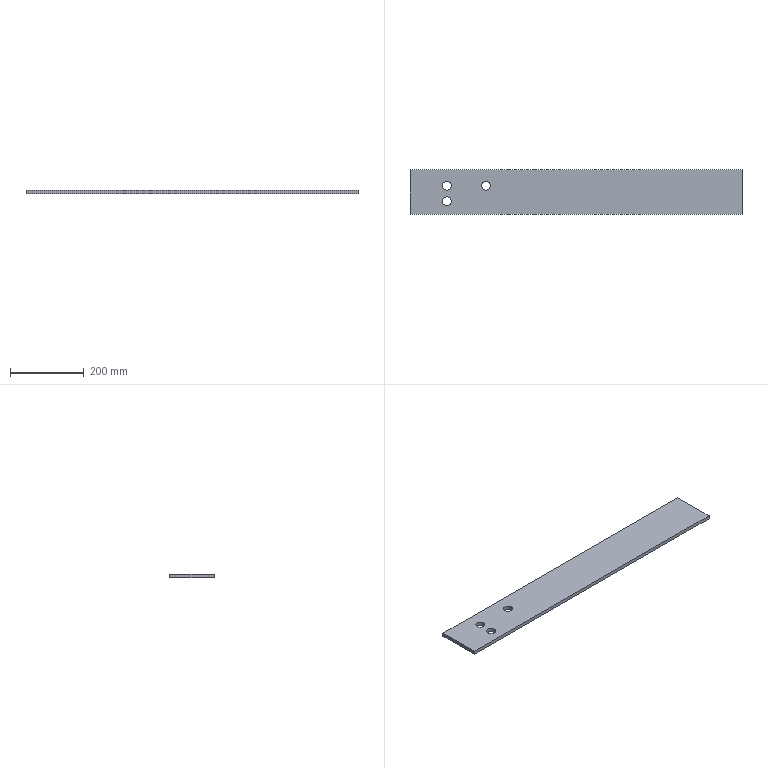Part | STEP file | zhiheceban2 | 1 solid | 9 faces | box 900 x 120 x 10 mm | volume 1066428 mm3 | plane 6 | cylinder 3 | commonest cylinder face diameters 24 x3
STEP:
#1=CARTESIAN_POINT('',(0.,0.,0.));
#2=DIRECTION('',(0.,0.,1.));
#3=DIRECTION('',(1.,0.,0.));
#4=AXIS2_PLACEMENT_3D('',#1,#2,#3);
#5=CARTESIAN_POINT('',(450.,-60.,-5.));
#6=VERTEX_POINT('',#5);
#7=CARTESIAN_POINT('',(450.,60.,-5.));
#8=VERTEX_POINT('',#7);
#9=CARTESIAN_POINT('',(450.,60.,-5.));
#10=DIRECTION('',(0.,1.,0.));
#11=VECTOR('',#10,1.);
#12=LINE('',#9,#11);
#13=CARTESIAN_POINT('',(450.,60.,5.));
#14=DIRECTION('',(-1.,0.,0.));
#15=DIRECTION('',(0.,0.,1.));
#16=AXIS2_PLACEMENT_3D('',#13,#14,#15);
#17=PLANE('',#16);
#18=CARTESIAN_POINT('',(-10.,0.));
#19=DIRECTION('',(0.,1.));
#20=VECTOR('',#19,1.);
#21=LINE('',#18,#20);
#22=(GEOMETRIC_REPRESENTATION_CONTEXT(2)PARAMETRIC_REPRESENTATION_CONTEXT()REPRESENTATION_CONTEXT('',''));
#23=DEFINITIONAL_REPRESENTATION('',(#21),#22);
#24=PCURVE('',#17,#23);
#25=CARTESIAN_POINT('',(0.,0.,-5.));
#26=DIRECTION('',(0.,0.,1.));
#27=DIRECTION('',(1.,0.,0.));
#28=AXIS2_PLACEMENT_3D('',#25,#26,#27);
#29=PLANE('',#28);
#30=CARTESIAN_POINT('',(450.,60.));
#31=DIRECTION('',(0.,1.));
#32=VECTOR('',#31,1.);
#33=LINE('',#30,#32);
#34=(GEOMETRIC_REPRESENTATION_CONTEXT(2)PARAMETRIC_REPRESENTATION_CONTEXT()REPRESENTATION_CONTEXT('',''));
#35=DEFINITIONAL_REPRESENTATION('',(#33),#34);
#36=PCURVE('',#29,#35);
#37=SURFACE_CURVE('',#12,(#24,#36),.PCURVE_S1.);
#38=EDGE_CURVE('',#6,#8,#37,.T.);
#39=ORIENTED_EDGE('',*,*,#38,.T.);
#40=CARTESIAN_POINT('',(450.,60.,5.));
#41=VERTEX_POINT('',#40);
#42=CARTESIAN_POINT('',(450.,60.,5.));
#43=DIRECTION('',(0.,0.,-1.));
#44=VECTOR('',#43,1.);
#45=LINE('',#42,#44);
#46=CARTESIAN_POINT('',(0.,0.));
#47=DIRECTION('',(-1.,0.));
#48=VECTOR('',#47,1.);
#49=LINE('',#46,#48);
#50=(GEOMETRIC_REPRESENTATION_CONTEXT(2)PARAMETRIC_REPRESENTATION_CONTEXT()REPRESENTATION_CONTEXT('',''));
#51=DEFINITIONAL_REPRESENTATION('',(#49),#50);
#52=PCURVE('',#17,#51);
#53=CARTESIAN_POINT('',(-450.,60.,5.));
#54=DIRECTION('',(0.,-1.,0.));
#55=DIRECTION('',(0.,0.,-1.));
#56=AXIS2_PLACEMENT_3D('',#53,#54,#55);
#57=PLANE('',#56);
#58=CARTESIAN_POINT('',(0.,900.));
#59=DIRECTION('',(1.,0.));
#60=VECTOR('',#59,1.);
#61=LINE('',#58,#60);
#62=(GEOMETRIC_REPRESENTATION_CONTEXT(2)PARAMETRIC_REPRESENTATION_CONTEXT()REPRESENTATION_CONTEXT('',''));
#63=DEFINITIONAL_REPRESENTATION('',(#61),#62);
#64=PCURVE('',#57,#63);
#65=SURFACE_CURVE('',#45,(#52,#64),.PCURVE_S1.);
#66=EDGE_CURVE('',#41,#8,#65,.T.);
#67=ORIENTED_EDGE('',*,*,#66,.F.);
#68=CARTESIAN_POINT('',(450.,-60.,5.));
#69=VERTEX_POINT('',#68);
#70=CARTESIAN_POINT('',(450.,60.,5.));
#71=DIRECTION('',(0.,1.,0.));
#72=VECTOR('',#71,1.);
#73=LINE('',#70,#72);
#74=CARTESIAN_POINT('',(0.,0.));
#75=DIRECTION('',(0.,1.));
#76=VECTOR('',#75,1.);
#77=LINE('',#74,#76);
#78=(GEOMETRIC_REPRESENTATION_CONTEXT(2)PARAMETRIC_REPRESENTATION_CONTEXT()REPRESENTATION_CONTEXT('',''));
#79=DEFINITIONAL_REPRESENTATION('',(#77),#78);
#80=PCURVE('',#17,#79);
#81=CARTESIAN_POINT('',(0.,0.,5.));
#82=DIRECTION('',(0.,0.,1.));
#83=DIRECTION('',(1.,0.,0.));
#84=AXIS2_PLACEMENT_3D('',#81,#82,#83);
#85=PLANE('',#84);
#86=CARTESIAN_POINT('',(450.,60.));
#87=DIRECTION('',(0.,1.));
#88=VECTOR('',#87,1.);
#89=LINE('',#86,#88);
#90=(GEOMETRIC_REPRESENTATION_CONTEXT(2)PARAMETRIC_REPRESENTATION_CONTEXT()REPRESENTATION_CONTEXT('',''));
#91=DEFINITIONAL_REPRESENTATION('',(#89),#90);
#92=PCURVE('',#85,#91);
#93=SURFACE_CURVE('',#73,(#80,#92),.PCURVE_S1.);
#94=EDGE_CURVE('',#69,#41,#93,.T.);
#95=ORIENTED_EDGE('',*,*,#94,.F.);
#96=CARTESIAN_POINT('',(450.,-60.,5.));
#97=DIRECTION('',(0.,0.,-1.));
#98=VECTOR('',#97,1.);
#99=LINE('',#96,#98);
#100=CARTESIAN_POINT('',(0.,-120.));
#101=DIRECTION('',(-1.,0.));
#102=VECTOR('',#101,1.);
#103=LINE('',#100,#102);
#104=(GEOMETRIC_REPRESENTATION_CONTEXT(2)PARAMETRIC_REPRESENTATION_CONTEXT()REPRESENTATION_CONTEXT('',''));
#105=DEFINITIONAL_REPRESENTATION('',(#103),#104);
#106=PCURVE('',#17,#105);
#107=CARTESIAN_POINT('',(-450.,-60.,5.));
#108=DIRECTION('',(0.,1.,0.));
#109=DIRECTION('',(0.,0.,1.));
#110=AXIS2_PLACEMENT_3D('',#107,#108,#109);
#111=PLANE('',#110);
#112=CARTESIAN_POINT('',(0.,900.));
#113=DIRECTION('',(-1.,0.));
#114=VECTOR('',#113,1.);
#115=LINE('',#112,#114);
#116=(GEOMETRIC_REPRESENTATION_CONTEXT(2)PARAMETRIC_REPRESENTATION_CONTEXT()REPRESENTATION_CONTEXT('',''));
#117=DEFINITIONAL_REPRESENTATION('',(#115),#116);
#118=PCURVE('',#111,#117);
#119=SURFACE_CURVE('',#99,(#106,#118),.PCURVE_S1.);
#120=EDGE_CURVE('',#69,#6,#119,.T.);
#121=ORIENTED_EDGE('',*,*,#120,.T.);
#122=EDGE_LOOP('',(#39,#67,#95,#121));
#123=FACE_BOUND('',#122,.T.);
#124=ADVANCED_FACE('',(#123),#17,.F.);
#125=CARTESIAN_POINT('',(-450.,60.,-5.));
#126=VERTEX_POINT('',#125);
#127=CARTESIAN_POINT('',(-450.,60.,-5.));
#128=DIRECTION('',(-1.,0.,0.));
#129=VECTOR('',#128,1.);
#130=LINE('',#127,#129);
#131=CARTESIAN_POINT('',(10.,0.));
#132=DIRECTION('',(0.,-1.));
#133=VECTOR('',#132,1.);
#134=LINE('',#131,#133);
#135=(GEOMETRIC_REPRESENTATION_CONTEXT(2)PARAMETRIC_REPRESENTATION_CONTEXT()REPRESENTATION_CONTEXT('',''));
#136=DEFINITIONAL_REPRESENTATION('',(#134),#135);
#137=PCURVE('',#57,#136);
#138=CARTESIAN_POINT('',(-450.,60.));
#139=DIRECTION('',(-1.,0.));
#140=VECTOR('',#139,1.);
#141=LINE('',#138,#140);
#142=(GEOMETRIC_REPRESENTATION_CONTEXT(2)PARAMETRIC_REPRESENTATION_CONTEXT()REPRESENTATION_CONTEXT('',''));
#143=DEFINITIONAL_REPRESENTATION('',(#141),#142);
#144=PCURVE('',#29,#143);
#145=SURFACE_CURVE('',#130,(#137,#144),.PCURVE_S1.);
#146=EDGE_CURVE('',#8,#126,#145,.T.);
#147=ORIENTED_EDGE('',*,*,#146,.T.);
#148=CARTESIAN_POINT('',(-450.,60.,5.));
#149=VERTEX_POINT('',#148);
#150=CARTESIAN_POINT('',(-450.,60.,5.));
#151=DIRECTION('',(0.,0.,-1.));
#152=VECTOR('',#151,1.);
#153=LINE('',#150,#152);
#154=CARTESIAN_POINT('',(0.,0.));
#155=DIRECTION('',(1.,0.));
#156=VECTOR('',#155,1.);
#157=LINE('',#154,#156);
#158=(GEOMETRIC_REPRESENTATION_CONTEXT(2)PARAMETRIC_REPRESENTATION_CONTEXT()REPRESENTATION_CONTEXT('',''));
#159=DEFINITIONAL_REPRESENTATION('',(#157),#158);
#160=PCURVE('',#57,#159);
#161=CARTESIAN_POINT('',(-450.,60.,5.));
#162=DIRECTION('',(1.,0.,0.));
#163=DIRECTION('',(0.,0.,-1.));
#164=AXIS2_PLACEMENT_3D('',#161,#162,#163);
#165=PLANE('',#164);
#166=CARTESIAN_POINT('',(0.,0.));
#167=DIRECTION('',(1.,0.));
#168=VECTOR('',#167,1.);
#169=LINE('',#166,#168);
#170=(GEOMETRIC_REPRESENTATION_CONTEXT(2)PARAMETRIC_REPRESENTATION_CONTEXT()REPRESENTATION_CONTEXT('',''));
#171=DEFINITIONAL_REPRESENTATION('',(#169),#170);
#172=PCURVE('',#165,#171);
#173=SURFACE_CURVE('',#153,(#160,#172),.PCURVE_S1.);
#174=EDGE_CURVE('',#149,#126,#173,.T.);
#175=ORIENTED_EDGE('',*,*,#174,.F.);
#176=CARTESIAN_POINT('',(-450.,60.,5.));
#177=DIRECTION('',(-1.,0.,0.));
#178=VECTOR('',#177,1.);
#179=LINE('',#176,#178);
#180=CARTESIAN_POINT('',(0.,0.));
#181=DIRECTION('',(0.,-1.));
#182=VECTOR('',#181,1.);
#183=LINE('',#180,#182);
#184=(GEOMETRIC_REPRESENTATION_CONTEXT(2)PARAMETRIC_REPRESENTATION_CONTEXT()REPRESENTATION_CONTEXT('',''));
#185=DEFINITIONAL_REPRESENTATION('',(#183),#184);
#186=PCURVE('',#57,#185);
#187=CARTESIAN_POINT('',(-450.,60.));
#188=DIRECTION('',(-1.,0.));
#189=VECTOR('',#188,1.);
#190=LINE('',#187,#189);
#191=(GEOMETRIC_REPRESENTATION_CONTEXT(2)PARAMETRIC_REPRESENTATION_CONTEXT()REPRESENTATION_CONTEXT('',''));
#192=DEFINITIONAL_REPRESENTATION('',(#190),#191);
#193=PCURVE('',#85,#192);
#194=SURFACE_CURVE('',#179,(#186,#193),.PCURVE_S1.);
#195=EDGE_CURVE('',#41,#149,#194,.T.);
#196=ORIENTED_EDGE('',*,*,#195,.F.);
#197=ORIENTED_EDGE('',*,*,#66,.T.);
#198=EDGE_LOOP('',(#147,#175,#196,#197));
#199=FACE_BOUND('',#198,.T.);
#200=ADVANCED_FACE('',(#199),#57,.F.);
#201=CARTESIAN_POINT('',(-450.,-60.,-5.));
#202=VERTEX_POINT('',#201);
#203=CARTESIAN_POINT('',(-450.,60.,-5.));
#204=DIRECTION('',(0.,-1.,0.));
#205=VECTOR('',#204,1.);
#206=LINE('',#203,#205);
#207=CARTESIAN_POINT('',(10.,0.));
#208=DIRECTION('',(0.,-1.));
#209=VECTOR('',#208,1.);
#210=LINE('',#207,#209);
#211=(GEOMETRIC_REPRESENTATION_CONTEXT(2)PARAMETRIC_REPRESENTATION_CONTEXT()REPRESENTATION_CONTEXT('',''));
#212=DEFINITIONAL_REPRESENTATION('',(#210),#211);
#213=PCURVE('',#165,#212);
#214=CARTESIAN_POINT('',(-450.,60.));
#215=DIRECTION('',(0.,-1.));
#216=VECTOR('',#215,1.);
#217=LINE('',#214,#216);
#218=(GEOMETRIC_REPRESENTATION_CONTEXT(2)PARAMETRIC_REPRESENTATION_CONTEXT()REPRESENTATION_CONTEXT('',''));
#219=DEFINITIONAL_REPRESENTATION('',(#217),#218);
#220=PCURVE('',#29,#219);
#221=SURFACE_CURVE('',#206,(#213,#220),.PCURVE_S1.);
#222=EDGE_CURVE('',#126,#202,#221,.T.);
#223=ORIENTED_EDGE('',*,*,#222,.T.);
#224=CARTESIAN_POINT('',(-450.,-60.,5.));
#225=VERTEX_POINT('',#224);
#226=CARTESIAN_POINT('',(-450.,-60.,5.));
#227=DIRECTION('',(0.,0.,-1.));
#228=VECTOR('',#227,1.);
#229=LINE('',#226,#228);
#230=CARTESIAN_POINT('',(0.,-120.));
#231=DIRECTION('',(1.,0.));
#232=VECTOR('',#231,1.);
#233=LINE('',#230,#232);
#234=(GEOMETRIC_REPRESENTATION_CONTEXT(2)PARAMETRIC_REPRESENTATION_CONTEXT()REPRESENTATION_CONTEXT('',''));
#235=DEFINITIONAL_REPRESENTATION('',(#233),#234);
#236=PCURVE('',#165,#235);
#237=CARTESIAN_POINT('',(0.,0.));
#238=DIRECTION('',(-1.,0.));
#239=VECTOR('',#238,1.);
#240=LINE('',#237,#239);
#241=(GEOMETRIC_REPRESENTATION_CONTEXT(2)PARAMETRIC_REPRESENTATION_CONTEXT()REPRESENTATION_CONTEXT('',''));
#242=DEFINITIONAL_REPRESENTATION('',(#240),#241);
#243=PCURVE('',#111,#242);
#244=SURFACE_CURVE('',#229,(#236,#243),.PCURVE_S1.);
#245=EDGE_CURVE('',#225,#202,#244,.T.);
#246=ORIENTED_EDGE('',*,*,#245,.F.);
#247=CARTESIAN_POINT('',(-450.,60.,5.));
#248=DIRECTION('',(0.,-1.,0.));
#249=VECTOR('',#248,1.);
#250=LINE('',#247,#249);
#251=CARTESIAN_POINT('',(0.,0.));
#252=DIRECTION('',(0.,-1.));
#253=VECTOR('',#252,1.);
#254=LINE('',#251,#253);
#255=(GEOMETRIC_REPRESENTATION_CONTEXT(2)PARAMETRIC_REPRESENTATION_CONTEXT()REPRESENTATION_CONTEXT('',''));
#256=DEFINITIONAL_REPRESENTATION('',(#254),#255);
#257=PCURVE('',#165,#256);
#258=CARTESIAN_POINT('',(-450.,60.));
#259=DIRECTION('',(0.,-1.));
#260=VECTOR('',#259,1.);
#261=LINE('',#258,#260);
#262=(GEOMETRIC_REPRESENTATION_CONTEXT(2)PARAMETRIC_REPRESENTATION_CONTEXT()REPRESENTATION_CONTEXT('',''));
#263=DEFINITIONAL_REPRESENTATION('',(#261),#262);
#264=PCURVE('',#85,#263);
#265=SURFACE_CURVE('',#250,(#257,#264),.PCURVE_S1.);
#266=EDGE_CURVE('',#149,#225,#265,.T.);
#267=ORIENTED_EDGE('',*,*,#266,.F.);
#268=ORIENTED_EDGE('',*,*,#174,.T.);
#269=EDGE_LOOP('',(#223,#246,#267,#268));
#270=FACE_BOUND('',#269,.T.);
#271=ADVANCED_FACE('',(#270),#165,.F.);
#272=CARTESIAN_POINT('',(-450.,-60.,-5.));
#273=DIRECTION('',(1.,0.,0.));
#274=VECTOR('',#273,1.);
#275=LINE('',#272,#274);
#276=CARTESIAN_POINT('',(-10.,0.));
#277=DIRECTION('',(0.,1.));
#278=VECTOR('',#277,1.);
#279=LINE('',#276,#278);
#280=(GEOMETRIC_REPRESENTATION_CONTEXT(2)PARAMETRIC_REPRESENTATION_CONTEXT()REPRESENTATION_CONTEXT('',''));
#281=DEFINITIONAL_REPRESENTATION('',(#279),#280);
#282=PCURVE('',#111,#281);
#283=CARTESIAN_POINT('',(-450.,-60.));
#284=DIRECTION('',(1.,0.));
#285=VECTOR('',#284,1.);
#286=LINE('',#283,#285);
#287=(GEOMETRIC_REPRESENTATION_CONTEXT(2)PARAMETRIC_REPRESENTATION_CONTEXT()REPRESENTATION_CONTEXT('',''));
#288=DEFINITIONAL_REPRESENTATION('',(#286),#287);
#289=PCURVE('',#29,#288);
#290=SURFACE_CURVE('',#275,(#282,#289),.PCURVE_S1.);
#291=EDGE_CURVE('',#202,#6,#290,.T.);
#292=ORIENTED_EDGE('',*,*,#291,.T.);
#293=ORIENTED_EDGE('',*,*,#120,.F.);
#294=CARTESIAN_POINT('',(-450.,-60.,5.));
#295=DIRECTION('',(1.,0.,0.));
#296=VECTOR('',#295,1.);
#297=LINE('',#294,#296);
#298=CARTESIAN_POINT('',(0.,0.));
#299=DIRECTION('',(0.,1.));
#300=VECTOR('',#299,1.);
#301=LINE('',#298,#300);
#302=(GEOMETRIC_REPRESENTATION_CONTEXT(2)PARAMETRIC_REPRESENTATION_CONTEXT()REPRESENTATION_CONTEXT('',''));
#303=DEFINITIONAL_REPRESENTATION('',(#301),#302);
#304=PCURVE('',#111,#303);
#305=CARTESIAN_POINT('',(-450.,-60.));
#306=DIRECTION('',(1.,0.));
#307=VECTOR('',#306,1.);
#308=LINE('',#305,#307);
#309=(GEOMETRIC_REPRESENTATION_CONTEXT(2)PARAMETRIC_REPRESENTATION_CONTEXT()REPRESENTATION_CONTEXT('',''));
#310=DEFINITIONAL_REPRESENTATION('',(#308),#309);
#311=PCURVE('',#85,#310);
#312=SURFACE_CURVE('',#297,(#304,#311),.PCURVE_S1.);
#313=EDGE_CURVE('',#225,#69,#312,.T.);
#314=ORIENTED_EDGE('',*,*,#313,.F.);
#315=ORIENTED_EDGE('',*,*,#245,.T.);
#316=EDGE_LOOP('',(#292,#293,#314,#315));
#317=FACE_BOUND('',#316,.T.);
#318=ADVANCED_FACE('',(#317),#111,.F.);
#319=CARTESIAN_POINT('',(-338.,17.,5.));
#320=VERTEX_POINT('',#319);
#321=CARTESIAN_POINT('',(-350.,17.,5.));
#322=DIRECTION('',(0.,0.,1.));
#323=DIRECTION('',(1.,0.,0.));
#324=AXIS2_PLACEMENT_3D('',#321,#322,#323);
#325=CIRCLE('',#324,12.);
#326=CARTESIAN_POINT('',(-350.,17.));
#327=DIRECTION('',(1.,0.));
#328=AXIS2_PLACEMENT_2D('',#326,#327);
#329=CIRCLE('',#328,12.);
#330=(GEOMETRIC_REPRESENTATION_CONTEXT(2)PARAMETRIC_REPRESENTATION_CONTEXT()REPRESENTATION_CONTEXT('',''));
#331=DEFINITIONAL_REPRESENTATION('',(#329),#330);
#332=PCURVE('',#85,#331);
#333=CARTESIAN_POINT('',(-350.,17.,-5.));
#334=DIRECTION('',(0.,0.,1.));
#335=DIRECTION('',(1.,0.,0.));
#336=AXIS2_PLACEMENT_3D('',#333,#334,#335);
#337=CYLINDRICAL_SURFACE('',#336,12.);
#338=CARTESIAN_POINT('',(0.,10.));
#339=DIRECTION('',(1.,0.));
#340=VECTOR('',#339,1.);
#341=LINE('',#338,#340);
#342=(GEOMETRIC_REPRESENTATION_CONTEXT(2)PARAMETRIC_REPRESENTATION_CONTEXT()REPRESENTATION_CONTEXT('',''));
#343=DEFINITIONAL_REPRESENTATION('',(#341),#342);
#344=PCURVE('',#337,#343);
#345=SURFACE_CURVE('',#325,(#332,#344),.PCURVE_S1.);
#346=EDGE_CURVE('',#320,#320,#345,.T.);
#347=ORIENTED_EDGE('',*,*,#346,.F.);
#348=EDGE_LOOP('',(#347));
#349=FACE_BOUND('',#348,.T.);
#350=CARTESIAN_POINT('',(-338.,-25.,5.));
#351=VERTEX_POINT('',#350);
#352=CARTESIAN_POINT('',(-350.,-25.,5.));
#353=DIRECTION('',(0.,0.,1.));
#354=DIRECTION('',(1.,0.,0.));
#355=AXIS2_PLACEMENT_3D('',#352,#353,#354);
#356=CIRCLE('',#355,12.);
#357=CARTESIAN_POINT('',(-350.,-25.));
#358=DIRECTION('',(1.,0.));
#359=AXIS2_PLACEMENT_2D('',#357,#358);
#360=CIRCLE('',#359,12.);
#361=(GEOMETRIC_REPRESENTATION_CONTEXT(2)PARAMETRIC_REPRESENTATION_CONTEXT()REPRESENTATION_CONTEXT('',''));
#362=DEFINITIONAL_REPRESENTATION('',(#360),#361);
#363=PCURVE('',#85,#362);
#364=CARTESIAN_POINT('',(-350.,-25.,-5.));
#365=DIRECTION('',(0.,0.,1.));
#366=DIRECTION('',(1.,0.,0.));
#367=AXIS2_PLACEMENT_3D('',#364,#365,#366);
#368=CYLINDRICAL_SURFACE('',#367,12.);
#369=CARTESIAN_POINT('',(0.,10.));
#370=DIRECTION('',(1.,0.));
#371=VECTOR('',#370,1.);
#372=LINE('',#369,#371);
#373=(GEOMETRIC_REPRESENTATION_CONTEXT(2)PARAMETRIC_REPRESENTATION_CONTEXT()REPRESENTATION_CONTEXT('',''));
#374=DEFINITIONAL_REPRESENTATION('',(#372),#373);
#375=PCURVE('',#368,#374);
#376=SURFACE_CURVE('',#356,(#363,#375),.PCURVE_S1.);
#377=EDGE_CURVE('',#351,#351,#376,.T.);
#378=ORIENTED_EDGE('',*,*,#377,.F.);
#379=EDGE_LOOP('',(#378));
#380=FACE_BOUND('',#379,.T.);
#381=CARTESIAN_POINT('',(-232.046,17.,5.));
#382=VERTEX_POINT('',#381);
#383=CARTESIAN_POINT('',(-244.046,17.,5.));
#384=DIRECTION('',(0.,0.,1.));
#385=DIRECTION('',(1.,0.,0.));
#386=AXIS2_PLACEMENT_3D('',#383,#384,#385);
#387=CIRCLE('',#386,12.);
#388=CARTESIAN_POINT('',(-244.046,17.));
#389=DIRECTION('',(1.,0.));
#390=AXIS2_PLACEMENT_2D('',#388,#389);
#391=CIRCLE('',#390,12.);
#392=(GEOMETRIC_REPRESENTATION_CONTEXT(2)PARAMETRIC_REPRESENTATION_CONTEXT()REPRESENTATION_CONTEXT('',''));
#393=DEFINITIONAL_REPRESENTATION('',(#391),#392);
#394=PCURVE('',#85,#393);
#395=CARTESIAN_POINT('',(-244.046,17.,-5.));
#396=DIRECTION('',(0.,0.,1.));
#397=DIRECTION('',(1.,0.,0.));
#398=AXIS2_PLACEMENT_3D('',#395,#396,#397);
#399=CYLINDRICAL_SURFACE('',#398,12.);
#400=CARTESIAN_POINT('',(0.,10.));
#401=DIRECTION('',(1.,0.));
#402=VECTOR('',#401,1.);
#403=LINE('',#400,#402);
#404=(GEOMETRIC_REPRESENTATION_CONTEXT(2)PARAMETRIC_REPRESENTATION_CONTEXT()REPRESENTATION_CONTEXT('',''));
#405=DEFINITIONAL_REPRESENTATION('',(#403),#404);
#406=PCURVE('',#399,#405);
#407=SURFACE_CURVE('',#387,(#394,#406),.PCURVE_S1.);
#408=EDGE_CURVE('',#382,#382,#407,.T.);
#409=ORIENTED_EDGE('',*,*,#408,.F.);
#410=EDGE_LOOP('',(#409));
#411=FACE_BOUND('',#410,.T.);
#412=ORIENTED_EDGE('',*,*,#94,.T.);
#413=ORIENTED_EDGE('',*,*,#195,.T.);
#414=ORIENTED_EDGE('',*,*,#266,.T.);
#415=ORIENTED_EDGE('',*,*,#313,.T.);
#416=EDGE_LOOP('',(#412,#413,#414,#415));
#417=FACE_BOUND('',#416,.T.);
#418=ADVANCED_FACE('',(#349,#380,#411,#417),#85,.T.);
#419=CARTESIAN_POINT('',(-338.,17.,-5.));
#420=VERTEX_POINT('',#419);
#421=CARTESIAN_POINT('',(-350.,17.,-5.));
#422=DIRECTION('',(0.,0.,1.));
#423=DIRECTION('',(1.,0.,0.));
#424=AXIS2_PLACEMENT_3D('',#421,#422,#423);
#425=CIRCLE('',#424,12.);
#426=CARTESIAN_POINT('',(-350.,17.));
#427=DIRECTION('',(1.,0.));
#428=AXIS2_PLACEMENT_2D('',#426,#427);
#429=CIRCLE('',#428,12.);
#430=(GEOMETRIC_REPRESENTATION_CONTEXT(2)PARAMETRIC_REPRESENTATION_CONTEXT()REPRESENTATION_CONTEXT('',''));
#431=DEFINITIONAL_REPRESENTATION('',(#429),#430);
#432=PCURVE('',#29,#431);
#433=CARTESIAN_POINT('',(0.,0.));
#434=DIRECTION('',(1.,0.));
#435=VECTOR('',#434,1.);
#436=LINE('',#433,#435);
#437=(GEOMETRIC_REPRESENTATION_CONTEXT(2)PARAMETRIC_REPRESENTATION_CONTEXT()REPRESENTATION_CONTEXT('',''));
#438=DEFINITIONAL_REPRESENTATION('',(#436),#437);
#439=PCURVE('',#337,#438);
#440=SURFACE_CURVE('',#425,(#432,#439),.PCURVE_S1.);
#441=EDGE_CURVE('',#420,#420,#440,.T.);
#442=ORIENTED_EDGE('',*,*,#441,.T.);
#443=EDGE_LOOP('',(#442));
#444=FACE_BOUND('',#443,.T.);
#445=CARTESIAN_POINT('',(-338.,-25.,-5.));
#446=VERTEX_POINT('',#445);
#447=CARTESIAN_POINT('',(-350.,-25.,-5.));
#448=DIRECTION('',(0.,0.,1.));
#449=DIRECTION('',(1.,0.,0.));
#450=AXIS2_PLACEMENT_3D('',#447,#448,#449);
#451=CIRCLE('',#450,12.);
#452=CARTESIAN_POINT('',(-350.,-25.));
#453=DIRECTION('',(1.,0.));
#454=AXIS2_PLACEMENT_2D('',#452,#453);
#455=CIRCLE('',#454,12.);
#456=(GEOMETRIC_REPRESENTATION_CONTEXT(2)PARAMETRIC_REPRESENTATION_CONTEXT()REPRESENTATION_CONTEXT('',''));
#457=DEFINITIONAL_REPRESENTATION('',(#455),#456);
#458=PCURVE('',#29,#457);
#459=CARTESIAN_POINT('',(0.,0.));
#460=DIRECTION('',(1.,0.));
#461=VECTOR('',#460,1.);
#462=LINE('',#459,#461);
#463=(GEOMETRIC_REPRESENTATION_CONTEXT(2)PARAMETRIC_REPRESENTATION_CONTEXT()REPRESENTATION_CONTEXT('',''));
#464=DEFINITIONAL_REPRESENTATION('',(#462),#463);
#465=PCURVE('',#368,#464);
#466=SURFACE_CURVE('',#451,(#458,#465),.PCURVE_S1.);
#467=EDGE_CURVE('',#446,#446,#466,.T.);
#468=ORIENTED_EDGE('',*,*,#467,.T.);
#469=EDGE_LOOP('',(#468));
#470=FACE_BOUND('',#469,.T.);
#471=CARTESIAN_POINT('',(-232.046,17.,-5.));
#472=VERTEX_POINT('',#471);
#473=CARTESIAN_POINT('',(-244.046,17.,-5.));
#474=DIRECTION('',(0.,0.,1.));
#475=DIRECTION('',(1.,0.,0.));
#476=AXIS2_PLACEMENT_3D('',#473,#474,#475);
#477=CIRCLE('',#476,12.);
#478=CARTESIAN_POINT('',(-244.046,17.));
#479=DIRECTION('',(1.,0.));
#480=AXIS2_PLACEMENT_2D('',#478,#479);
#481=CIRCLE('',#480,12.);
#482=(GEOMETRIC_REPRESENTATION_CONTEXT(2)PARAMETRIC_REPRESENTATION_CONTEXT()REPRESENTATION_CONTEXT('',''));
#483=DEFINITIONAL_REPRESENTATION('',(#481),#482);
#484=PCURVE('',#29,#483);
#485=CARTESIAN_POINT('',(0.,0.));
#486=DIRECTION('',(1.,0.));
#487=VECTOR('',#486,1.);
#488=LINE('',#485,#487);
#489=(GEOMETRIC_REPRESENTATION_CONTEXT(2)PARAMETRIC_REPRESENTATION_CONTEXT()REPRESENTATION_CONTEXT('',''));
#490=DEFINITIONAL_REPRESENTATION('',(#488),#489);
#491=PCURVE('',#399,#490);
#492=SURFACE_CURVE('',#477,(#484,#491),.PCURVE_S1.);
#493=EDGE_CURVE('',#472,#472,#492,.T.);
#494=ORIENTED_EDGE('',*,*,#493,.T.);
#495=EDGE_LOOP('',(#494));
#496=FACE_BOUND('',#495,.T.);
#497=ORIENTED_EDGE('',*,*,#38,.F.);
#498=ORIENTED_EDGE('',*,*,#291,.F.);
#499=ORIENTED_EDGE('',*,*,#222,.F.);
#500=ORIENTED_EDGE('',*,*,#146,.F.);
#501=EDGE_LOOP('',(#497,#498,#499,#500));
#502=FACE_BOUND('',#501,.T.);
#503=ADVANCED_FACE('',(#444,#470,#496,#502),#29,.F.);
#504=ORIENTED_EDGE('',*,*,#493,.T.);
#505=CARTESIAN_POINT('',(-232.046,17.,-5.));
#506=CARTESIAN_POINT('',(-232.046,17.,5.));
#507=B_SPLINE_CURVE_WITH_KNOTS('',1,(#505,#506),.UNSPECIFIED.,.F.,.F.,(2,2),(0.,10.),.PIECEWISE_BEZIER_KNOTS.);
#508=CARTESIAN_POINT('',(6.283,0.));
#509=DIRECTION('',(0.,1.));
#510=VECTOR('',#509,1.);
#511=LINE('',#508,#510);
#512=(GEOMETRIC_REPRESENTATION_CONTEXT(2)PARAMETRIC_REPRESENTATION_CONTEXT()REPRESENTATION_CONTEXT('',''));
#513=DEFINITIONAL_REPRESENTATION('',(#511),#512);
#514=PCURVE('',#399,#513);
#515=CARTESIAN_POINT('',(0.,0.));
#516=DIRECTION('',(0.,1.));
#517=VECTOR('',#516,1.);
#518=LINE('',#515,#517);
#519=(GEOMETRIC_REPRESENTATION_CONTEXT(2)PARAMETRIC_REPRESENTATION_CONTEXT()REPRESENTATION_CONTEXT('',''));
#520=DEFINITIONAL_REPRESENTATION('',(#518),#519);
#521=PCURVE('',#399,#520);
#522=SEAM_CURVE('',#507,(#514,#521),.PCURVE_S1.);
#523=EDGE_CURVE('',#472,#382,#522,.T.);
#524=ORIENTED_EDGE('',*,*,#523,.T.);
#525=ORIENTED_EDGE('',*,*,#408,.F.);
#526=ORIENTED_EDGE('',*,*,#523,.F.);
#527=EDGE_LOOP('',(#504,#524,#525,#526));
#528=FACE_BOUND('',#527,.F.);
#529=ADVANCED_FACE('',(#528),#399,.F.);
#530=ORIENTED_EDGE('',*,*,#467,.T.);
#531=CARTESIAN_POINT('',(-338.,-25.,-5.));
#532=CARTESIAN_POINT('',(-338.,-25.,5.));
#533=B_SPLINE_CURVE_WITH_KNOTS('',1,(#531,#532),.UNSPECIFIED.,.F.,.F.,(2,2),(0.,10.),.PIECEWISE_BEZIER_KNOTS.);
#534=CARTESIAN_POINT('',(6.283,0.));
#535=DIRECTION('',(0.,1.));
#536=VECTOR('',#535,1.);
#537=LINE('',#534,#536);
#538=(GEOMETRIC_REPRESENTATION_CONTEXT(2)PARAMETRIC_REPRESENTATION_CONTEXT()REPRESENTATION_CONTEXT('',''));
#539=DEFINITIONAL_REPRESENTATION('',(#537),#538);
#540=PCURVE('',#368,#539);
#541=CARTESIAN_POINT('',(0.,0.));
#542=DIRECTION('',(0.,1.));
#543=VECTOR('',#542,1.);
#544=LINE('',#541,#543);
#545=(GEOMETRIC_REPRESENTATION_CONTEXT(2)PARAMETRIC_REPRESENTATION_CONTEXT()REPRESENTATION_CONTEXT('',''));
#546=DEFINITIONAL_REPRESENTATION('',(#544),#545);
#547=PCURVE('',#368,#546);
#548=SEAM_CURVE('',#533,(#540,#547),.PCURVE_S1.);
#549=EDGE_CURVE('',#446,#351,#548,.T.);
#550=ORIENTED_EDGE('',*,*,#549,.T.);
#551=ORIENTED_EDGE('',*,*,#377,.F.);
#552=ORIENTED_EDGE('',*,*,#549,.F.);
#553=EDGE_LOOP('',(#530,#550,#551,#552));
#554=FACE_BOUND('',#553,.F.);
#555=ADVANCED_FACE('',(#554),#368,.F.);
#556=ORIENTED_EDGE('',*,*,#441,.T.);
#557=CARTESIAN_POINT('',(-338.,17.,-5.));
#558=CARTESIAN_POINT('',(-338.,17.,5.));
#559=B_SPLINE_CURVE_WITH_KNOTS('',1,(#557,#558),.UNSPECIFIED.,.F.,.F.,(2,2),(0.,10.),.PIECEWISE_BEZIER_KNOTS.);
#560=CARTESIAN_POINT('',(6.283,0.));
#561=DIRECTION('',(0.,1.));
#562=VECTOR('',#561,1.);
#563=LINE('',#560,#562);
#564=(GEOMETRIC_REPRESENTATION_CONTEXT(2)PARAMETRIC_REPRESENTATION_CONTEXT()REPRESENTATION_CONTEXT('',''));
#565=DEFINITIONAL_REPRESENTATION('',(#563),#564);
#566=PCURVE('',#337,#565);
#567=CARTESIAN_POINT('',(0.,0.));
#568=DIRECTION('',(0.,1.));
#569=VECTOR('',#568,1.);
#570=LINE('',#567,#569);
#571=(GEOMETRIC_REPRESENTATION_CONTEXT(2)PARAMETRIC_REPRESENTATION_CONTEXT()REPRESENTATION_CONTEXT('',''));
#572=DEFINITIONAL_REPRESENTATION('',(#570),#571);
#573=PCURVE('',#337,#572);
#574=SEAM_CURVE('',#559,(#566,#573),.PCURVE_S1.);
#575=EDGE_CURVE('',#420,#320,#574,.T.);
#576=ORIENTED_EDGE('',*,*,#575,.T.);
#577=ORIENTED_EDGE('',*,*,#346,.F.);
#578=ORIENTED_EDGE('',*,*,#575,.F.);
#579=EDGE_LOOP('',(#556,#576,#577,#578));
#580=FACE_BOUND('',#579,.F.);
#581=ADVANCED_FACE('',(#580),#337,.F.);
#582=CLOSED_SHELL('',(#124,#200,#271,#318,#418,#503,#529,#555,#581));
#583=MANIFOLD_SOLID_BREP('',#582);
#584=(LENGTH_UNIT()NAMED_UNIT(*)SI_UNIT(.MILLI.,.METRE.));
#585=UNCERTAINTY_MEASURE_WITH_UNIT(LENGTH_MEASURE(0.000002),#584,'','');
#586=(NAMED_UNIT(*)PLANE_ANGLE_UNIT()SI_UNIT($,.RADIAN.));
#587=(NAMED_UNIT(*)SI_UNIT($,.STERADIAN.)SOLID_ANGLE_UNIT());
#588=(GEOMETRIC_REPRESENTATION_CONTEXT(3)GLOBAL_UNCERTAINTY_ASSIGNED_CONTEXT((#585))GLOBAL_UNIT_ASSIGNED_CONTEXT((#584,#586,#587))REPRESENTATION_CONTEXT('',''));
#589=ADVANCED_BREP_SHAPE_REPRESENTATION('',(#4,#583),#588);